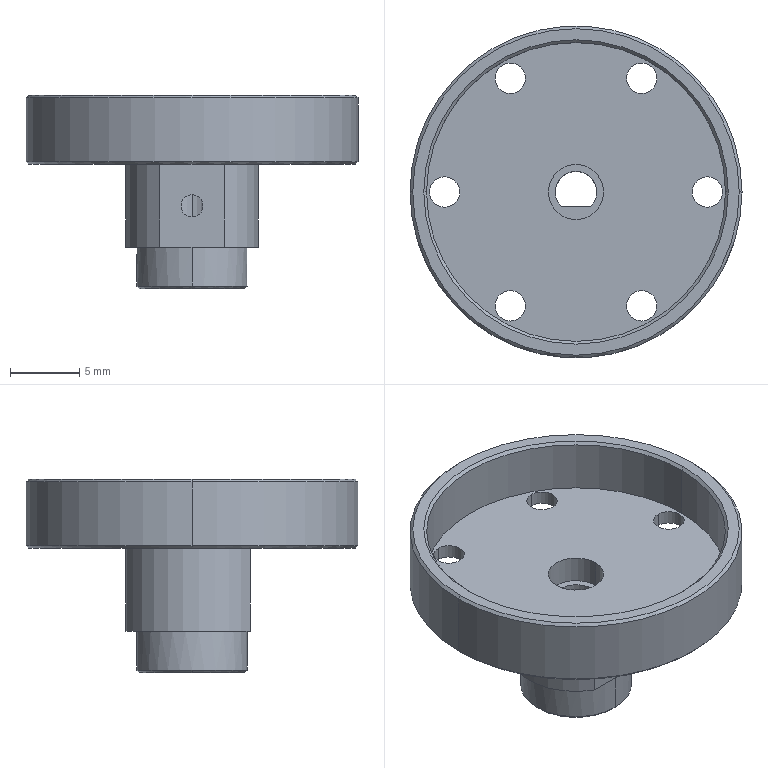NC program | NX | posted with a generic post | part box 24 x 24 x 14 mm
Lines 1 to 1709 of 3647, first 1603 of 1689 lines:
N10 G17 G21 G94 G90
(FLOOR_WALL_COPY , TOOL : D80)
N12 T19 M6
N14 G54
N16 G17 G0 G90 X-55. Y0. S6500 M3
N18 G43 Z30. H19
N20 Z8.
N22 G94 G1 Z5. F1500.
N24 X-52.
N26 X52.
N28 X55.
N30 Z8.
N32 G0 Z30.
N34 X-55.
N36 Z7.
N38 G1 Z4.
N40 X-52.
N42 X52.
N44 X55.
N46 Z7.
N48 G0 Z30.
N50 X-55.
N52 Z6.
N54 G1 Z3.
N56 X-52.
N58 X52.
N60 X55.
N62 Z6.
N64 G0 Z30.
N66 X-55.
N68 Z5.
N70 G1 Z2.
N72 X-52.
N74 X52.
N76 X55.
N78 Z5.
N80 G0 Z30.
N82 X-55.
N84 Z4.
N86 G1 Z1.
N88 X-52.
N90 X52.
N92 X55.
N94 Z4.
N96 G0 Z30.
N98 X-55.
N100 Z3.
N102 G1 Z0.
N104 X-52.
N106 X52.
N108 X55.
N110 Z3.
N112 G0 Z30.
N114 M5
(FLOOR_WALL_2 , TOOL : D10)
N116 T15 M6
N118 G54
N120 G17 G0 G90 X-18.446 Y-1.412 S9500 M3
N122 G43 Z30. H15
N124 Z1.1
N126 G94 G1 Z-0.4 F1000.
N128 X-17.5 Y-0.866
N130 G3 X-17. Y0. R1.
N132 G2 X0. Y17. R17. F2000.
N134 X-17. Y0. R-17.
N136 G1 X-12.
N138 G2 X0. Y12. R12.
N140 X-12. Y0. R-12.
N142 G1 X-9.9
N144 G2 X4.793 Y-8.663 R-9.9
N146 G1 X3.641 Y-9.3
N148 X-3.641
N150 X-4.793 Y-8.663
N152 G2 X-9.9 Y0. R9.9
N154 G3 X-10.4 Y0.866 R1.
N156 G1 Z1.1
N158 G0 X-18.446 Y-1.412 Z0.6
N160 G1 Z-0.9 F1000.
N162 X-17.5 Y-0.866
N164 G3 X-17. Y0. R1.
N166 G2 X0. Y17. R17. F2000.
N168 X-17. Y0. R-17.
N170 G1 X-12.
N172 G2 X0. Y12. R12.
N174 X-12. Y0. R-12.
N176 G1 X-9.9
N178 G2 X4.793 Y-8.663 R-9.9
N180 G1 X3.641 Y-9.3
N182 X-3.641
N184 X-4.793 Y-8.663
N186 G2 X-9.9 Y0. R9.9
N188 G3 X-10.4 Y0.866 R1.
N190 G1 Z0.6
N192 G0 X-18.446 Y-1.412 Z0.1
N194 G1 Z-1.4 F1000.
N196 X-17.5 Y-0.866
N198 G3 X-17. Y0. R1.
N200 G2 X0. Y17. R17. F2000.
N202 X-17. Y0. R-17.
N204 G1 X-12.
N206 G2 X0. Y12. R12.
N208 X-12. Y0. R-12.
N210 G1 X-9.9
N212 G2 X4.793 Y-8.663 R-9.9
N214 G1 X3.641 Y-9.3
N216 X-3.641
N218 X-4.793 Y-8.663
N220 G2 X-9.9 Y0. R9.9
N222 G3 X-10.4 Y0.866 R1.
N224 G1 Z0.1
N226 G0 X-18.446 Y-1.412 Z-0.4
N228 G1 Z-1.9 F1000.
N230 X-17.5 Y-0.866
N232 G3 X-17. Y0. R1.
N234 G2 X0. Y17. R17. F2000.
N236 X-17. Y0. R-17.
N238 G1 X-12.
N240 G2 X0. Y12. R12.
N242 X-12. Y0. R-12.
N244 G1 X-9.9
N246 G2 X4.793 Y-8.663 R-9.9
N248 G1 X3.641 Y-9.3
N250 X-3.641
N252 X-4.793 Y-8.663
N254 G2 X-9.9 Y0. R9.9
N256 G3 X-10.4 Y0.866 R1.
N258 G1 Z-0.4
N260 G0 X-18.446 Y-1.412 Z-0.9
N262 G1 Z-2.4 F1000.
N264 X-17.5 Y-0.866
N266 G3 X-17. Y0. R1.
N268 G2 X0. Y17. R17. F2000.
N270 X-17. Y0. R-17.
N272 G1 X-12.
N274 G2 X0. Y12. R12.
N276 X-12. Y0. R-12.
N278 G1 X-9.9
N280 G2 X4.793 Y-8.663 R-9.9
N282 G1 X3.641 Y-9.3
N284 X-3.641
N286 X-4.793 Y-8.663
N288 G2 X-9.9 Y0. R9.9
N290 G3 X-10.4 Y0.866 R1.
N292 G1 Z-0.9
N294 G0 X-18.446 Y-1.412 Z-1.4
N296 G1 Z-2.9 F1000.
N298 X-17.5 Y-0.866
N300 G3 X-17. Y0. R1.
N302 G2 X0. Y17. R17. F2000.
N304 X-17. Y0. R-17.
N306 G1 X-12.
N308 G2 X0. Y12. R12.
N310 X-12. Y0. R-12.
N312 G1 X-9.9
N314 G2 X4.793 Y-8.663 R-9.9
N316 G1 X3.641 Y-9.3
N318 X-3.641
N320 X-4.793 Y-8.663
N322 G2 X-9.9 Y0. R9.9
N324 G3 X-10.4 Y0.866 R1.
N326 G1 Z-1.4
N328 G0 X-18.446 Y-1.412 Z-1.9
N330 G1 Z-3.4 F1000.
N332 X-17.5 Y-0.866
N334 G3 X-17. Y0. R1.
N336 G2 X0. Y17. R17. F2000.
N338 X-17. Y0. R-17.
N340 G1 X-12.
N342 G2 X0. Y12. R12.
N344 X-12. Y0. R-12.
N346 G1 X-9.9
N348 G2 X4.793 Y-8.663 R-9.9
N350 G1 X3.641 Y-9.3
N352 X-3.641
N354 X-4.793 Y-8.663
N356 G2 X-9.9 Y0. R9.9
N358 G3 X-10.4 Y0.866 R1.
N360 G1 Z-1.9
N362 G0 X-18.446 Y-1.412 Z-2.4
N364 G1 Z-3.9 F1000.
N366 X-17.5 Y-0.866
N368 G3 X-17. Y0. R1.
N370 G2 X0. Y17. R17. F2000.
N372 X-17. Y0. R-17.
N374 G1 X-12.
N376 G2 X0. Y12. R12.
N378 X-12. Y0. R-12.
N380 G1 X-9.9
N382 G2 X4.793 Y-8.663 R-9.9
N384 G1 X3.641 Y-9.3
N386 X-3.641
N388 X-4.793 Y-8.663
N390 G2 X-9.9 Y0. R9.9
N392 G3 X-10.4 Y0.866 R1.
N394 G1 Z-2.4
N396 G0 X-18.446 Y-1.412 Z-2.9
N398 G1 Z-4.4 F1000.
N400 X-17.5 Y-0.866
N402 G3 X-17. Y0. R1.
N404 G2 X0. Y17. R17. F2000.
N406 X-17. Y0. R-17.
N408 G1 X-12.
N410 G2 X0. Y12. R12.
N412 X-12. Y0. R-12.
N414 G1 X-9.9
N416 G2 X4.793 Y-8.663 R-9.9
N418 G1 X3.641 Y-9.3
N420 X-3.641
N422 X-4.793 Y-8.663
N424 G2 X-9.9 Y0. R9.9
N426 G3 X-10.4 Y0.866 R1.
N428 G1 Z-2.9
N430 G0 X-18.446 Y-1.412 Z-3.4
N432 G1 Z-4.9 F1000.
N434 X-17.5 Y-0.866
N436 G3 X-17. Y0. R1.
N438 G2 X0. Y17. R17. F2000.
N440 X-17. Y0. R-17.
N442 G1 X-12.
N444 G2 X0. Y12. R12.
N446 X-12. Y0. R-12.
N448 G1 X-9.9
N450 G2 X4.793 Y-8.663 R-9.9
N452 G1 X3.641 Y-9.3
N454 X-3.641
N456 X-4.793 Y-8.663
N458 G2 X-9.9 Y0. R9.9
N460 G3 X-10.4 Y0.866 R1.
N462 G1 Z-3.4
N464 G0 X-18.446 Y-1.412 Z-3.9
N466 G1 Z-5.4 F1000.
N468 X-17.5 Y-0.866
N470 G3 X-17. Y0. R1.
N472 G2 X0. Y17. R17. F2000.
N474 X-17. Y0. R-17.
N476 G1 X-12.
N478 G2 X0. Y12. R12.
N480 X-12. Y0. R-12.
N482 G1 X-9.9
N484 G2 X4.793 Y-8.663 R-9.9
N486 G1 X3.641 Y-9.3
N488 X-3.641
N490 X-4.793 Y-8.663
N492 G2 X-9.9 Y0. R9.9
N494 G3 X-10.4 Y0.866 R1.
N496 G1 Z-3.9
N498 G0 X-18.446 Y-1.412 Z-4.4
N500 G1 Z-5.9 F1000.
N502 X-17.5 Y-0.866
N504 G3 X-17. Y0. R1.
N506 G2 X0. Y17. R17. F2000.
N508 X-17. Y0. R-17.
N510 G1 X-12.
N512 G2 X0. Y12. R12.
N514 X-12. Y0. R-12.
N516 G1 X-9.9
N518 G2 X4.793 Y-8.663 R-9.9
N520 G1 X3.641 Y-9.3
N522 X-3.641
N524 X-4.793 Y-8.663
N526 G2 X-9.9 Y0. R9.9
N528 G3 X-10.4 Y0.866 R1.
N530 G1 Z-4.4
N532 G0 X-18.446 Y-1.412 Z-4.9
N534 G1 Z-6.4 F1000.
N536 X-17.5 Y-0.866
N538 G3 X-17. Y0. R1.
N540 G2 X0. Y17. R17. F2000.
N542 X-17. Y0. R-17.
N544 G1 X-12.
N546 G2 X0. Y12. R12.
N548 X-12. Y0. R-12.
N550 G1 X-9.9
N552 G2 X4.793 Y-8.663 R-9.9
N554 G1 X3.641 Y-9.3
N556 X-3.641
N558 X-4.793 Y-8.663
N560 G2 X-9.9 Y0. R9.9
N562 G3 X-10.4 Y0.866 R1.
N564 G1 Z-4.9
N566 G0 X-18.446 Y-1.412 Z-5.4
N568 G1 Z-6.9 F1000.
N570 X-17.5 Y-0.866
N572 G3 X-17. Y0. R1.
N574 G2 X0. Y17. R17. F2000.
N576 X-17. Y0. R-17.
N578 G1 X-12.
N580 G2 X0. Y12. R12.
N582 X-12. Y0. R-12.
N584 G1 X-9.9
N586 G2 X4.793 Y-8.663 R-9.9
N588 G1 X3.641 Y-9.3
N590 X-3.641
N592 X-4.793 Y-8.663
N594 G2 X-9.9 Y0. R9.9
N596 G3 X-10.4 Y0.866 R1.
N598 G1 Z-5.4
N600 G0 X-18.446 Y-1.412 Z-5.9
N602 G1 Z-7.4 F1000.
N604 X-17.5 Y-0.866
N606 G3 X-17. Y0. R1.
N608 G2 X0. Y17. R17. F2000.
N610 X-17. Y0. R-17.
N612 G1 X-12.
N614 G2 X0. Y12. R12.
N616 X-12. Y0. R-12.
N618 G1 X-9.9
N620 G2 X4.793 Y-8.663 R-9.9
N622 G1 X3.641 Y-9.3
N624 X-3.641
N626 X-4.793 Y-8.663
N628 G2 X-9.9 Y0. R9.9
N630 G3 X-10.4 Y0.866 R1.
N632 G1 Z-5.9
N634 G0 X-18.446 Y-1.412 Z-6.4
N636 G1 Z-7.9 F1000.
N638 X-17.5 Y-0.866
N640 G3 X-17. Y0. R1.
N642 G2 X0. Y17. R17. F2000.
N644 X-17. Y0. R-17.
N646 G1 X-12.
N648 G2 X0. Y12. R12.
N650 X-12. Y0. R-12.
N652 G1 X-9.9
N654 G2 X4.793 Y-8.663 R-9.9
N656 G1 X3.641 Y-9.3
N658 X-3.641
N660 X-4.793 Y-8.663
N662 G2 X-9.9 Y0. R9.9
N664 G3 X-10.4 Y0.866 R1.
N666 G1 Z-6.4
N668 G0 X-18.446 Y-1.412 Z-6.9
N670 G1 Z-8.4 F1000.
N672 X-17.5 Y-0.866
N674 G3 X-17. Y0. R1.
N676 G2 X0. Y17. R17. F2000.
N678 X-17. Y0. R-17.
N680 G1 X-12.
N682 G2 X0. Y12. R12.
N684 X-12. Y0. R-12.
N686 G1 X-9.9
N688 G2 X4.793 Y-8.663 R-9.9
N690 G1 X3.641 Y-9.3
N692 X-3.641
N694 X-4.793 Y-8.663
N696 G2 X-9.9 Y0. R9.9
N698 G3 X-10.4 Y0.866 R1.
N700 G1 Z-6.9
N702 G0 X-18.446 Y-1.412 Z-7.4
N704 G1 Z-8.9 F1000.
N706 X-17.5 Y-0.866
N708 G3 X-17. Y0. R1.
N710 G2 X0. Y17. R17. F2000.
N712 X-17. Y0. R-17.
N714 G1 X-12.
N716 G2 X0. Y12. R12.
N718 X-12. Y0. R-12.
N720 G1 X-9.9
N722 G2 X4.793 Y-8.663 R-9.9
N724 G1 X3.641 Y-9.3
N726 X-3.641
N728 X-4.793 Y-8.663
N730 G2 X-9.9 Y0. R9.9
N732 G3 X-10.4 Y0.866 R1.
N734 G1 Z-7.4
N736 G0 Z30.
(FLOOR_WALL_2_COPY , TOOL : D10)
N738 X-10.508 Y-1.39
N740 Z1.1
N742 G1 Z-0.4 F1000.
N744 X-9.6 Y-0.866
N746 G3 X-9.1 Y0. R1.
N748 G2 X0. Y9.1 R9.1 F2000.
N750 X-9.1 Y0. R-9.1
N752 G3 X-9.6 Y0.866 R1.
N754 G1 X-10.508 Y1.39
N756 Z1.1
N758 G0 Y-1.39 Z0.6
N760 G1 Z-0.9 F1000.
N762 X-9.6 Y-0.866
N764 G3 X-9.1 Y0. R1.
N766 G2 X0. Y9.1 R9.1 F2000.
N768 X-9.1 Y0. R-9.1
N770 G3 X-9.6 Y0.866 R1.
N772 G1 X-10.508 Y1.39
N774 Z0.6
N776 G0 Y-1.39 Z0.1
N778 G1 Z-1.4 F1000.
N780 X-9.6 Y-0.866
N782 G3 X-9.1 Y0. R1.
N784 G2 X0. Y9.1 R9.1 F2000.
N786 X-9.1 Y0. R-9.1
N788 G3 X-9.6 Y0.866 R1.
N790 G1 X-10.508 Y1.39
N792 Z0.1
N794 G0 Y-1.39 Z-0.4
N796 G1 Z-1.9 F1000.
N798 X-9.6 Y-0.866
N800 G3 X-9.1 Y0. R1.
N802 G2 X0. Y9.1 R9.1 F2000.
N804 X-9.1 Y0. R-9.1
N806 G3 X-9.6 Y0.866 R1.
N808 G1 X-10.508 Y1.39
N810 Z-0.4
N812 G0 Y-1.39 Z-0.9
N814 G1 Z-2.4 F1000.
N816 X-9.6 Y-0.866
N818 G3 X-9.1 Y0. R1.
N820 G2 X0. Y9.1 R9.1 F2000.
N822 X-9.1 Y0. R-9.1
N824 G3 X-9.6 Y0.866 R1.
N826 G1 X-10.508 Y1.39
N828 Z-0.9
N830 G0 Y-1.39 Z-1.4
N832 G1 Z-2.9 F1000.
N834 X-9.6 Y-0.866
N836 G3 X-9.1 Y0. R1.
N838 G2 X0. Y9.1 R9.1 F2000.
N840 X-9.1 Y0. R-9.1
N842 G3 X-9.6 Y0.866 R1.
N844 G1 X-10.508 Y1.39
N846 Z-1.4
N848 G0 Z30.
N850 M5
(FLOOR_WALL_1_COPY , TOOL : D10JING)
N852 T14 M6
N854 G54
N856 G17 G0 G90 X2.021 Y-12.2 S9500 M3
N858 G43 Z30. H14
N860 Z-6.
N862 G94 G1 Z-9. F1250.
N864 X0.866 Y-10.2
N866 G3 X0. Y-9.7 R1.
N868 G1 X-3.615
N870 G2 X-3.857 Y-9.638 R0.5
N872 G1 X-4.986 Y-9.013
N874 G2 X4.986 Y-9.013 R-10.3
N876 G1 X3.857 Y-9.638
N878 G2 X3.615 Y-9.7 R0.5
N880 G1 X0.
N882 X0.866
N884 G3 X0. Y-9.2 R1.
N886 G1 X-3.615
N888 X-4.744 Y-8.575
N890 G2 X4.744 Y-8.575 R-9.8
N892 G1 X3.615 Y-9.2
N894 X0.
N896 G3 X-0.866 Y-9.7 R1.
N898 G1 X-2.598 Y-12.7
N900 Z-6.
N902 G0 Z30.
N904 M5
(DRILLING , TOOL : D6A45)
N906 T01 M6
N908 G54
N910 G17 G0 G90 X2.75 Y0. S5000 M3
N912 G43 Z30. H1
N914 G94 G81 G98 Z-0.725 F350. R3.
N916 X-2.75
N918 G80
N920 G0 X-2.75 Y0. Z30.
(DRILLING_COPY , TOOL : D6A45)
N922 X9.5
N924 G81 Z-10.2 F350. R-6.
N926 X4.75 Y-8.227
N928 X-4.75
N930 X-9.5 Y0.
N932 X-4.75 Y8.227
N934 X4.75
N936 G80
N938 G0 X4.75 Y8.227 Z30.
N940 M5
(DRILLING_COPY_1 , TOOL : 1.25ZT)
N942 T17 M6
N944 G54
N946 G17 G0 G90 X2.75 Y0. S2000 M3
N948 G43 Z30. H17
N950 G94 G83 G98 Z-4.626 F120. Q1. R3.
N952 X-2.75
N954 G80
N956 G0 X-2.75 Y0. Z30.
N958 M5
(DRILLING_COPY_1_COPY , TOOL : 2.2ZT)
N960 T18 M6
N962 G54
N964 G17 G0 G90 X-4.75 Y8.227 S2000 M3
N966 G43 Z30. H18
N968 G94 G83 G98 Z-12.161 F120. Q1. R-6.
N970 Y-8.227
N972 X9.5 Y0.
N974 X4.75 Y-8.227
N976 X-9.5 Y0.
N978 X4.75 Y8.227
N980 G80
N982 G0 X4.75 Y8.227 Z30.
N984 M5
(ZLEVEL_PROFILE , TOOL : D2)
N986 T24 M6
N988 G54
N990 G17 G0 G90 X-0.272 Y0.298 S9500 M3
N992 G43 Z30. H24
N994 Z0.5
N996 G94 G1 X-0.35 Y0.213 Z0.494 F1000.
N998 X-0.379 Y0.128 Z0.489
N1000 X-0.389 Y0.05 Z0.485
N1002 X0.389 Z0.444
N1004 X0.379 Y0.127 Z0.44
N1006 X0.351 Y0.212 Z0.436
N1008 X0.238 Y0.334 Z0.427
N1010 X0.086 Y0.401 Z0.418
N1012 X-0.094 Y0.399 Z0.409
N1014 X-0.241 Y0.332 Z0.4
N1016 X-0.35 Y0.213 Z0.392
N1018 X-0.379 Y0.128 Z0.387
N1020 X-0.389 Y0.05 Z0.383
N1022 X0.389 Z0.342
N1024 X0.379 Y0.127 Z0.338
N1026 X0.351 Y0.212 Z0.333
N1028 X0.238 Y0.334 Z0.325
N1030 X0.086 Y0.401 Z0.316
N1032 X-0.094 Y0.399 Z0.307
N1034 X-0.241 Y0.332 Z0.298
N1036 X-0.35 Y0.213 Z0.29
N1038 X-0.379 Y0.128 Z0.285
N1040 X-0.389 Y0.05 Z0.281
N1042 X0.389 Z0.24
N1044 X0.379 Y0.127 Z0.236
N1046 X0.351 Y0.212 Z0.231
N1048 X0.238 Y0.334 Z0.223
N1050 X0.086 Y0.401 Z0.214
N1052 X-0.094 Y0.399 Z0.204
N1054 X-0.241 Y0.332 Z0.196
N1056 X-0.35 Y0.213 Z0.187
N1058 X-0.379 Y0.128 Z0.183
N1060 X-0.389 Y0.05 Z0.179
N1062 X0.389 Z0.138
N1064 X0.379 Y0.127 Z0.134
N1066 X0.351 Y0.212 Z0.129
N1068 X0.238 Y0.334 Z0.12
N1070 X0.086 Y0.401 Z0.112
N1072 X-0.094 Y0.399 Z0.102
N1074 X-0.241 Y0.332 Z0.094
N1076 X-0.35 Y0.213 Z0.085
N1078 X-0.379 Y0.128 Z0.081
N1080 X-0.389 Y0.05 Z0.077
N1082 X0.389 Z0.036
N1084 X0.379 Y0.127 Z0.032
N1086 X0.351 Y0.212 Z0.027
N1088 X0.238 Y0.334 Z0.018
N1090 X0.086 Y0.401 Z0.01
N1092 X-0.094 Y0.399 Z0.
N1094 X-0.241 Y0.332 Z-0.008
N1096 X-0.35 Y0.213 Z-0.017
N1098 X-0.379 Y0.128 Z-0.022
N1100 X-0.389 Y0.05 Z-0.026
N1102 X0.389 Z-0.066
N1104 X0.379 Y0.127 Z-0.07
N1106 X0.351 Y0.212 Z-0.075
N1108 X0.238 Y0.334 Z-0.084
N1110 X0.086 Y0.401 Z-0.093
N1112 X-0.094 Y0.399 Z-0.102
N1114 X-0.241 Y0.332 Z-0.11
N1116 X-0.35 Y0.213 Z-0.119
N1118 X-0.379 Y0.128 Z-0.124
N1120 X-0.389 Y0.05 Z-0.128
N1122 X0. Z-0.148
N1124 X0.389
N1126 X0.379 Y0.127
N1128 G3 X-0.379 Y0.128 R0.4
N1130 G1 X-0.389 Y0.05
N1132 X0.
N1134 X0.181 Z-0.167
N1136 X0.387 Y0.06 Z-0.181
N1138 X0.379 Y0.107 Z-0.185
N1140 X0.359 Y0.157 Z-0.194
N1142 X0.332 Y0.21 Z-0.204
N1144 X0.224 Y0.324 Z-0.222
N1146 X0.172 Y0.354 Z-0.228
N1148 X0.145 Y0.366 Z-0.231
N1150 X0.117 Y0.375 Z-0.235
N1152 X0.059 Y0.388 Z-0.241
N1154 X-0.012 Y0.394 Z-0.248
N1156 X-0.071 Y0.387 Z-0.254
N1158 X-0.117 Y0.375 Z-0.259
N1160 X-0.184 Y0.347 Z-0.267
N1162 X-0.235 Y0.317 Z-0.273
N1164 X-0.269 Y0.286 Z-0.278
N1166 X-0.327 Y0.218 Z-0.287
N1168 X-0.374 Y0.142 Z-0.296
N1170 X-0.379 Y0.128
N1172 X-0.389 Y0.05
N1174 X0.
N1176 X0.181 Z-0.315
N1178 X0.387 Y0.06 Z-0.329
N1180 X0.379 Y0.107 Z-0.333
N1182 X0.359 Y0.157 Z-0.342
N1184 X0.332 Y0.21 Z-0.352
N1186 X0.224 Y0.324 Z-0.37
N1188 X0.172 Y0.354 Z-0.377
N1190 X0.145 Y0.366 Z-0.38
N1192 X0.117 Y0.375 Z-0.383
N1194 X0.059 Y0.388 Z-0.389
N1196 X-0.012 Y0.394 Z-0.396
N1198 X-0.071 Y0.387 Z-0.402
N1200 X-0.117 Y0.375 Z-0.407
N1202 X-0.184 Y0.347 Z-0.415
N1204 X-0.235 Y0.317 Z-0.421
N1206 X-0.269 Y0.286 Z-0.426
N1208 X-0.327 Y0.218 Z-0.435
N1210 X-0.374 Y0.142 Z-0.444
N1212 X-0.379 Y0.128
N1214 X-0.389 Y0.05
N1216 X0.
N1218 X0.181 Z-0.463
N1220 X0.387 Y0.06 Z-0.477
N1222 X0.379 Y0.107 Z-0.481
N1224 X0.359 Y0.157 Z-0.491
N1226 X0.332 Y0.21 Z-0.5
N1228 X0.224 Y0.324 Z-0.519
N1230 X0.172 Y0.354 Z-0.525
N1232 X0.145 Y0.366 Z-0.528
N1234 X0.117 Y0.375 Z-0.531
N1236 X0.059 Y0.388 Z-0.537
N1238 X-0.012 Y0.394 Z-0.544
N1240 X-0.071 Y0.387 Z-0.551
N1242 X-0.117 Y0.375 Z-0.556
N1244 X-0.184 Y0.347 Z-0.563
N1246 X-0.235 Y0.317 Z-0.569
N1248 X-0.269 Y0.286 Z-0.574
N1250 X-0.327 Y0.218 Z-0.583
N1252 X-0.374 Y0.142 Z-0.593
N1254 X-0.379 Y0.128
N1256 X-0.389 Y0.05
N1258 X0.
N1260 X0.181 Z-0.611
N1262 X0.387 Y0.06 Z-0.626
N1264 X0.379 Y0.107 Z-0.63
N1266 X0.359 Y0.157 Z-0.639
N1268 X0.332 Y0.21 Z-0.648
N1270 X0.224 Y0.324 Z-0.667
N1272 X0.172 Y0.354 Z-0.673
N1274 X0.145 Y0.366 Z-0.676
N1276 X0.117 Y0.375 Z-0.679
N1278 X0.059 Y0.388 Z-0.685
N1280 X-0.012 Y0.394 Z-0.693
N1282 X-0.071 Y0.387 Z-0.699
N1284 X-0.117 Y0.375 Z-0.704
N1286 X-0.184 Y0.347 Z-0.711
N1288 X-0.235 Y0.317 Z-0.717
N1290 X-0.269 Y0.286 Z-0.722
N1292 X-0.327 Y0.218 Z-0.731
N1294 X-0.374 Y0.142 Z-0.741
N1296 X-0.379 Y0.128
N1298 X-0.389 Y0.05
N1300 X0.
N1302 X0.181 Z-0.759
N1304 X0.387 Y0.06 Z-0.774
N1306 X0.379 Y0.107 Z-0.778
N1308 X0.359 Y0.157 Z-0.787
N1310 X0.332 Y0.21 Z-0.796
N1312 X0.224 Y0.324 Z-0.815
N1314 X0.172 Y0.354 Z-0.821
N1316 X0.145 Y0.366 Z-0.824
N1318 X0.117 Y0.375 Z-0.827
N1320 X0.059 Y0.388 Z-0.833
N1322 X-0.012 Y0.394 Z-0.841
N1324 X-0.071 Y0.387 Z-0.847
N1326 X-0.117 Y0.375 Z-0.852
N1328 X-0.184 Y0.347 Z-0.859
N1330 X-0.235 Y0.317 Z-0.866
N1332 X-0.269 Y0.286 Z-0.87
N1334 X-0.327 Y0.218 Z-0.88
N1336 X-0.374 Y0.142 Z-0.889
N1338 X-0.379 Y0.128
N1340 X-0.389 Y0.05
N1342 X0.
N1344 X0.181 Z-0.907
N1346 X0.387 Y0.06 Z-0.922
N1348 X0.379 Y0.107 Z-0.926
N1350 X0.359 Y0.157 Z-0.935
N1352 X0.332 Y0.21 Z-0.944
N1354 X0.224 Y0.324 Z-0.963
N1356 X0.172 Y0.354 Z-0.969
N1358 X0.145 Y0.366 Z-0.972
N1360 X0.117 Y0.375 Z-0.975
N1362 X0.059 Y0.388 Z-0.981
N1364 X-0.012 Y0.394 Z-0.989
N1366 X-0.071 Y0.387 Z-0.995
N1368 X-0.117 Y0.375 Z-1.
N1370 X-0.184 Y0.347 Z-1.008
N1372 X-0.235 Y0.317 Z-1.014
N1374 X-0.269 Y0.286 Z-1.019
N1376 X-0.327 Y0.218 Z-1.028
N1378 X-0.374 Y0.142 Z-1.037
N1380 X-0.379 Y0.128
N1382 X-0.389 Y0.05
N1384 X0.
N1386 X0.181 Z-1.056
N1388 X0.387 Y0.06 Z-1.07
N1390 X0.379 Y0.107 Z-1.074
N1392 X0.359 Y0.157 Z-1.083
N1394 X0.332 Y0.21 Z-1.092
N1396 X0.224 Y0.324 Z-1.111
N1398 X0.172 Y0.354 Z-1.117
N1400 X0.145 Y0.366 Z-1.12
N1402 X0.117 Y0.375 Z-1.123
N1404 X0.059 Y0.388 Z-1.13
N1406 X-0.012 Y0.394 Z-1.137
N1408 X-0.071 Y0.387 Z-1.143
N1410 X-0.117 Y0.375 Z-1.148
N1412 X-0.184 Y0.347 Z-1.156
N1414 X-0.235 Y0.317 Z-1.162
N1416 X-0.269 Y0.286 Z-1.167
N1418 X-0.327 Y0.218 Z-1.176
N1420 X-0.374 Y0.142 Z-1.185
N1422 X-0.379 Y0.128
N1424 X-0.389 Y0.05
N1426 X0.
N1428 X0.181 Z-1.204
N1430 X0.387 Y0.06 Z-1.218
N1432 X0.379 Y0.107 Z-1.222
N1434 X0.359 Y0.157 Z-1.231
N1436 X0.332 Y0.21 Z-1.241
N1438 X0.224 Y0.324 Z-1.259
N1440 X0.172 Y0.354 Z-1.265
N1442 X0.145 Y0.366 Z-1.268
N1444 X0.117 Y0.375 Z-1.272
N1446 X0.059 Y0.388 Z-1.278
N1448 X-0.012 Y0.394 Z-1.285
N1450 X-0.071 Y0.387 Z-1.291
N1452 X-0.117 Y0.375 Z-1.296
N1454 X-0.184 Y0.347 Z-1.304
N1456 X-0.235 Y0.317 Z-1.31
N1458 X-0.269 Y0.286 Z-1.315
N1460 X-0.327 Y0.218 Z-1.324
N1462 X-0.374 Y0.142 Z-1.333
N1464 X-0.379 Y0.128
N1466 X-0.389 Y0.05
N1468 X0.
N1470 X0.181 Z-1.352
N1472 X0.387 Y0.06 Z-1.366
N1474 X0.379 Y0.107 Z-1.37
N1476 X0.359 Y0.157 Z-1.379
N1478 X0.332 Y0.21 Z-1.389
N1480 X0.224 Y0.324 Z-1.407
N1482 X0.172 Y0.354 Z-1.414
N1484 X0.145 Y0.366 Z-1.417
N1486 X0.117 Y0.375 Z-1.42
N1488 X0.059 Y0.388 Z-1.426
N1490 X-0.012 Y0.394 Z-1.433
N1492 X-0.071 Y0.387 Z-1.439
N1494 X-0.117 Y0.375 Z-1.444
N1496 X-0.184 Y0.347 Z-1.452
N1498 X-0.235 Y0.317 Z-1.458
N1500 X-0.269 Y0.286 Z-1.463
N1502 X-0.327 Y0.218 Z-1.472
N1504 X-0.374 Y0.142 Z-1.481
N1506 X-0.379 Y0.128
N1508 X-0.389 Y0.05
N1510 X0.
N1512 X0.181 Z-1.5
N1514 X0.387 Y0.06 Z-1.514
N1516 X0.379 Y0.107 Z-1.518
N1518 X0.359 Y0.157 Z-1.528
N1520 X0.332 Y0.21 Z-1.537
N1522 X0.224 Y0.324 Z-1.556
N1524 X0.172 Y0.354 Z-1.562
N1526 X0.145 Y0.366 Z-1.565
N1528 X0.117 Y0.375 Z-1.568
N1530 X0.059 Y0.388 Z-1.574
N1532 X-0.012 Y0.394 Z-1.581
N1534 X-0.071 Y0.387 Z-1.588
N1536 X-0.117 Y0.375 Z-1.593
N1538 X-0.184 Y0.347 Z-1.6
N1540 X-0.235 Y0.317 Z-1.606
N1542 X-0.269 Y0.286 Z-1.611
N1544 X-0.327 Y0.218 Z-1.62
N1546 X-0.374 Y0.142 Z-1.63
N1548 X-0.379 Y0.128
N1550 X-0.389 Y0.05
N1552 X0.
N1554 X0.181 Z-1.648
N1556 X0.387 Y0.06 Z-1.663
N1558 X0.379 Y0.107 Z-1.667
N1560 X0.359 Y0.157 Z-1.676
N1562 X0.332 Y0.21 Z-1.685
N1564 X0.224 Y0.324 Z-1.704
N1566 X0.172 Y0.354 Z-1.71
N1568 X0.145 Y0.366 Z-1.713
N1570 X0.117 Y0.375 Z-1.716
N1572 X0.059 Y0.388 Z-1.722
N1574 X-0.012 Y0.394 Z-1.73
N1576 X-0.071 Y0.387 Z-1.736
N1578 X-0.117 Y0.375 Z-1.741
N1580 X-0.184 Y0.347 Z-1.748
N1582 X-0.235 Y0.317 Z-1.754
N1584 X-0.269 Y0.286 Z-1.759
N1586 X-0.327 Y0.218 Z-1.769
N1588 X-0.374 Y0.142 Z-1.778
N1590 X-0.379 Y0.128
N1592 X-0.389 Y0.05
N1594 X0.
N1596 X0.181 Z-1.796
N1598 X0.387 Y0.06 Z-1.811
N1600 X0.379 Y0.107 Z-1.815
N1602 X0.359 Y0.157 Z-1.824
N1604 X0.332 Y0.21 Z-1.833
N1606 X0.224 Y0.324 Z-1.852
N1608 X0.172 Y0.354 Z-1.858
N1610 X0.145 Y0.366 Z-1.861
N1612 X0.117 Y0.375 Z-1.864
N1614 X0.059 Y0.388 Z-1.87
N1616 X-0.012 Y0.394 Z-1.878
N1618 X-0.071 Y0.387 Z-1.884
N1620 X-0.117 Y0.375 Z-1.889
N1622 X-0.184 Y0.347 Z-1.896
N1624 X-0.235 Y0.317 Z-1.903
N1626 X-0.269 Y0.286 Z-1.907
N1628 X-0.327 Y0.218 Z-1.917
N1630 X-0.374 Y0.142 Z-1.926
N1632 X-0.379 Y0.128
N1634 X-0.389 Y0.05
N1636 X0.
N1638 X0.181 Z-1.944
N1640 X0.387 Y0.06 Z-1.959
N1642 X0.379 Y0.107 Z-1.963
N1644 X0.359 Y0.157 Z-1.972
N1646 X0.332 Y0.21 Z-1.981
N1648 X0.224 Y0.324 Z-2.
N1650 X0.172 Y0.354 Z-2.006
N1652 X0.145 Y0.366 Z-2.009
N1654 X0.117 Y0.375 Z-2.012
N1656 X0.059 Y0.388 Z-2.019
N1658 X-0.012 Y0.394 Z-2.026
N1660 X-0.071 Y0.387 Z-2.032
N1662 X-0.117 Y0.375 Z-2.037
N1664 X-0.184 Y0.347 Z-2.045
N1666 X-0.235 Y0.317 Z-2.051
N1668 X-0.269 Y0.286 Z-2.056
N1670 X-0.327 Y0.218 Z-2.065
N1672 X-0.374 Y0.142 Z-2.074
N1674 X-0.379 Y0.128
N1676 X-0.389 Y0.05
N1678 X0.
N1680 X0.181 Z-2.093
N1682 X0.387 Y0.06 Z-2.107
N1684 X0.379 Y0.107 Z-2.111
N1686 X0.359 Y0.157 Z-2.12
N1688 X0.332 Y0.21 Z-2.13
N1690 X0.224 Y0.324 Z-2.148
N1692 X0.172 Y0.354 Z-2.154
N1694 X0.145 Y0.366 Z-2.157
N1696 X0.117 Y0.375 Z-2.16
N1698 X0.059 Y0.388 Z-2.167
N1700 X-0.012 Y0.394 Z-2.174
N1702 X-0.071 Y0.387 Z-2.18
N1704 X-0.117 Y0.375 Z-2.185
N1706 X-0.184 Y0.347 Z-2.193
N1708 X-0.235 Y0.317 Z-2.199
N1710 X-0.269 Y0.286 Z-2.204
N1712 X-0.327 Y0.218 Z-2.213
N1714 X-0.374 Y0.142 Z-2.222
N1716 X-0.379 Y0.128
N1718 X-0.389 Y0.05
N1720 X0.
N1722 X0.181 Z-2.241
N1724 X0.387 Y0.06 Z-2.255
N1726 X0.379 Y0.107 Z-2.259
N1728 X0.359 Y0.157 Z-2.268
N1730 X0.332 Y0.21 Z-2.278
N1732 X0.224 Y0.324 Z-2.296
N1734 X0.172 Y0.354 Z-2.302
N1736 X0.145 Y0.366 Z-2.306
N1738 X0.117 Y0.375 Z-2.309
N1740 X0.059 Y0.388 Z-2.315
N1742 X-0.012 Y0.394 Z-2.322
N1744 X-0.071 Y0.387 Z-2.328
N1746 X-0.117 Y0.375 Z-2.333
N1748 X-0.184 Y0.347 Z-2.341
N1750 X-0.235 Y0.317 Z-2.347
N1752 X-0.269 Y0.286 Z-2.352
N1754 X-0.327 Y0.218 Z-2.361
N1756 X-0.374 Y0.142 Z-2.37
N1758 X-0.379 Y0.128
N1760 X-0.389 Y0.05
N1762 X0.
N1764 X0.181 Z-2.389
N1766 X0.387 Y0.06 Z-2.403
N1768 X0.379 Y0.107 Z-2.407
N1770 X0.359 Y0.157 Z-2.417
N1772 X0.332 Y0.21 Z-2.426
N1774 X0.224 Y0.324 Z-2.444
N1776 X0.172 Y0.354 Z-2.451
N1778 X0.145 Y0.366 Z-2.454
N1780 X0.117 Y0.375 Z-2.457
N1782 X0.059 Y0.388 Z-2.463
N1784 X-0.012 Y0.394 Z-2.47
N1786 X-0.071 Y0.387 Z-2.476
N1788 X-0.117 Y0.375 Z-2.481
N1790 X-0.184 Y0.347 Z-2.489
N1792 X-0.235 Y0.317 Z-2.495
N1794 X-0.269 Y0.286 Z-2.5
N1796 X-0.327 Y0.218 Z-2.509
N1798 X-0.374 Y0.142 Z-2.519
N1800 X-0.379 Y0.128
N1802 X-0.389 Y0.05
N1804 X0.
N1806 X0.181 Z-2.537
N1808 X0.387 Y0.06 Z-2.551
N1810 X0.379 Y0.107 Z-2.555
N1812 X0.359 Y0.157 Z-2.565
N1814 X0.332 Y0.21 Z-2.574
N1816 X0.224 Y0.324 Z-2.593
N1818 X0.172 Y0.354 Z-2.599
N1820 X0.145 Y0.366 Z-2.602
N1822 X0.117 Y0.375 Z-2.605
N1824 X0.059 Y0.388 Z-2.611
N1826 X-0.012 Y0.394 Z-2.618
N1828 X-0.071 Y0.387 Z-2.625
N1830 X-0.117 Y0.375 Z-2.63
N1832 X-0.184 Y0.347 Z-2.637
N1834 X-0.235 Y0.317 Z-2.643
N1836 X-0.269 Y0.286 Z-2.648
N1838 X-0.327 Y0.218 Z-2.657
N1840 X-0.374 Y0.142 Z-2.667
N1842 X-0.379 Y0.128
N1844 X-0.389 Y0.05
N1846 X0.
N1848 X0.181 Z-2.685
N1850 X0.387 Y0.06 Z-2.7
N1852 X0.379 Y0.107 Z-2.704
N1854 X0.359 Y0.157 Z-2.713
N1856 X0.332 Y0.21 Z-2.722
N1858 X0.224 Y0.324 Z-2.741
N1860 X0.172 Y0.354 Z-2.747
N1862 X0.145 Y0.366 Z-2.75
N1864 X0.117 Y0.375 Z-2.753
N1866 X0.059 Y0.388 Z-2.759
N1868 X-0.012 Y0.394 Z-2.767
N1870 X-0.071 Y0.387 Z-2.773
N1872 X-0.117 Y0.375 Z-2.778
N1874 X-0.184 Y0.347 Z-2.785
N1876 X-0.235 Y0.317 Z-2.791
N1878 X-0.269 Y0.286 Z-2.796
N1880 X-0.327 Y0.218 Z-2.806
N1882 X-0.374 Y0.142 Z-2.815
N1884 X-0.379 Y0.128
N1886 X-0.389 Y0.05
N1888 X0.
N1890 X0.181 Z-2.833
N1892 X0.387 Y0.06 Z-2.848
N1894 X0.379 Y0.107 Z-2.852
N1896 X0.359 Y0.157 Z-2.861
N1898 X0.332 Y0.21 Z-2.87
N1900 X0.224 Y0.324 Z-2.889
N1902 X0.172 Y0.354 Z-2.895
N1904 X0.145 Y0.366 Z-2.898
N1906 X0.117 Y0.375 Z-2.901
N1908 X0.059 Y0.388 Z-2.907
N1910 X-0.012 Y0.394 Z-2.915
N1912 X-0.071 Y0.387 Z-2.921
N1914 X-0.117 Y0.375 Z-2.926
N1916 X-0.184 Y0.347 Z-2.933
N1918 X-0.235 Y0.317 Z-2.94
N1920 X-0.269 Y0.286 Z-2.944
N1922 X-0.327 Y0.218 Z-2.954
N1924 X-0.374 Y0.142 Z-2.963
N1926 X-0.379 Y0.128
N1928 X-0.389 Y0.05
N1930 X0.
N1932 X0.181 Z-2.981
N1934 X0.387 Y0.06 Z-2.996
N1936 X0.379 Y0.107 Z-3.
N1938 X0.359 Y0.157 Z-3.009
N1940 X0.332 Y0.21 Z-3.018
N1942 X0.224 Y0.324 Z-3.037
N1944 X0.172 Y0.354 Z-3.043
N1946 X0.145 Y0.366 Z-3.046
N1948 X0.117 Y0.375 Z-3.049
N1950 X0.059 Y0.388 Z-3.056
N1952 X-0.012 Y0.394 Z-3.063
N1954 X-0.071 Y0.387 Z-3.069
N1956 X-0.117 Y0.375 Z-3.074
N1958 X-0.184 Y0.347 Z-3.082
N1960 X-0.235 Y0.317 Z-3.088
N1962 X-0.269 Y0.286 Z-3.093
N1964 X-0.327 Y0.218 Z-3.102
N1966 X-0.374 Y0.142 Z-3.111
N1968 X-0.379 Y0.128
N1970 X-0.389 Y0.05
N1972 X0.
N1974 X0.181 Z-3.13
N1976 X0.387 Y0.06 Z-3.144
N1978 X0.379 Y0.107 Z-3.148
N1980 X0.359 Y0.157 Z-3.157
N1982 X0.332 Y0.21 Z-3.167
N1984 X0.224 Y0.324 Z-3.185
N1986 X0.172 Y0.354 Z-3.191
N1988 X0.145 Y0.366 Z-3.194
N1990 X0.117 Y0.375 Z-3.198
N1992 X0.059 Y0.388 Z-3.204
N1994 X-0.012 Y0.394 Z-3.211
N1996 X-0.071 Y0.387 Z-3.217
N1998 X-0.117 Y0.375 Z-3.222
N2000 X-0.184 Y0.347 Z-3.23
N2002 X-0.235 Y0.317 Z-3.236
N2004 X-0.269 Y0.286 Z-3.241
N2006 X-0.327 Y0.218 Z-3.25
N2008 X-0.374 Y0.142 Z-3.259
N2010 X-0.379 Y0.128
N2012 X-0.389 Y0.05
N2014 X0.
N2016 X0.181 Z-3.278
N2018 X0.387 Y0.06 Z-3.292
N2020 X0.379 Y0.107 Z-3.296
N2022 X0.359 Y0.157 Z-3.305
N2024 X0.332 Y0.21 Z-3.315
N2026 X0.224 Y0.324 Z-3.333
N2028 X0.172 Y0.354 Z-3.339
N2030 X0.145 Y0.366 Z-3.343
N2032 X0.117 Y0.375 Z-3.346
N2034 X0.059 Y0.388 Z-3.352
N2036 X-0.012 Y0.394 Z-3.359
N2038 X-0.071 Y0.387 Z-3.365
N2040 X-0.117 Y0.375 Z-3.37
N2042 X-0.184 Y0.347 Z-3.378
N2044 X-0.235 Y0.317 Z-3.384
N2046 X-0.269 Y0.286 Z-3.389
N2048 X-0.327 Y0.218 Z-3.398
N2050 X-0.374 Y0.142 Z-3.407
N2052 X-0.379 Y0.128
N2054 X-0.389 Y0.05
N2056 X0.
N2058 X0.181 Z-3.426
N2060 X0.387 Y0.06 Z-3.44
N2062 X0.379 Y0.107 Z-3.444
N2064 X0.359 Y0.157 Z-3.454
N2066 X0.332 Y0.21 Z-3.463
N2068 X0.224 Y0.324 Z-3.481
N2070 X0.172 Y0.354 Z-3.488
N2072 X0.145 Y0.366 Z-3.491
N2074 X0.117 Y0.375 Z-3.494
N2076 X0.059 Y0.388 Z-3.5
N2078 X-0.012 Y0.394 Z-3.507
N2080 X-0.071 Y0.387 Z-3.514
N2082 X-0.117 Y0.375 Z-3.519
N2084 X-0.184 Y0.347 Z-3.526
N2086 X-0.235 Y0.317 Z-3.532
N2088 X-0.269 Y0.286 Z-3.537
N2090 X-0.327 Y0.218 Z-3.546
N2092 X-0.374 Y0.142 Z-3.556
N2094 X-0.379 Y0.128
N2096 X-0.389 Y0.05
N2098 X0.
N2100 X0.181 Z-3.574
N2102 X0.387 Y0.06 Z-3.588
N2104 X0.379 Y0.107 Z-3.592
N2106 X0.359 Y0.157 Z-3.602
N2108 X0.332 Y0.21 Z-3.611
N2110 X0.224 Y0.324 Z-3.63
N2112 X0.172 Y0.354 Z-3.636
N2114 X0.145 Y0.366 Z-3.639
N2116 X0.117 Y0.375 Z-3.642
N2118 X0.059 Y0.388 Z-3.648
N2120 X-0.012 Y0.394 Z-3.655
N2122 X-0.071 Y0.387 Z-3.662
N2124 X-0.117 Y0.375 Z-3.667
N2126 X-0.184 Y0.347 Z-3.674
N2128 X-0.235 Y0.317 Z-3.68
N2130 X-0.269 Y0.286 Z-3.685
N2132 X-0.327 Y0.218 Z-3.694
N2134 X-0.374 Y0.142 Z-3.704
N2136 X-0.379 Y0.128
N2138 X-0.389 Y0.05
N2140 X0.
N2142 X0.181 Z-3.722
N2144 X0.387 Y0.06 Z-3.737
N2146 X0.379 Y0.107 Z-3.741
N2148 X0.359 Y0.157 Z-3.75
N2150 X0.332 Y0.21 Z-3.759
N2152 X0.224 Y0.324 Z-3.778
N2154 X0.172 Y0.354 Z-3.784
N2156 X0.145 Y0.366 Z-3.787
N2158 X0.117 Y0.375 Z-3.79
N2160 X0.059 Y0.388 Z-3.796
N2162 X-0.012 Y0.394 Z-3.804
N2164 X-0.071 Y0.387 Z-3.81
N2166 X-0.117 Y0.375 Z-3.815
N2168 X-0.184 Y0.347 Z-3.822
N2170 X-0.235 Y0.317 Z-3.829
N2172 X-0.269 Y0.286 Z-3.833
N2174 X-0.327 Y0.218 Z-3.843
N2176 X-0.374 Y0.142 Z-3.852
N2178 X-0.379 Y0.128
N2180 X-0.389 Y0.05
N2182 X0.
N2184 X0.181 Z-3.87
N2186 X0.387 Y0.06 Z-3.885
N2188 X0.379 Y0.107 Z-3.889
N2190 X0.359 Y0.157 Z-3.898
N2192 X0.332 Y0.21 Z-3.907
N2194 X0.224 Y0.324 Z-3.926
N2196 X0.172 Y0.354 Z-3.932
N2198 X0.145 Y0.366 Z-3.935
N2200 X0.117 Y0.375 Z-3.938
N2202 X0.059 Y0.388 Z-3.944
N2204 X-0.012 Y0.394 Z-3.952
N2206 X-0.071 Y0.387 Z-3.958
N2208 X-0.117 Y0.375 Z-3.963
N2210 X-0.184 Y0.347 Z-3.97
N2212 X-0.235 Y0.317 Z-3.977
N2214 X-0.269 Y0.286 Z-3.981
N2216 X-0.327 Y0.218 Z-3.991
N2218 X-0.374 Y0.142 Z-4.
N2220 X-0.379 Y0.128
N2222 X-0.389 Y0.05
N2224 X0.
N2226 X0.181 Z-4.019
N2228 X0.387 Y0.06 Z-4.033
N2230 X0.379 Y0.107 Z-4.037
N2232 X0.359 Y0.157 Z-4.046
N2234 X0.332 Y0.21 Z-4.055
N2236 X0.224 Y0.324 Z-4.074
N2238 X0.172 Y0.354 Z-4.08
N2240 X0.145 Y0.366 Z-4.083
N2242 X0.117 Y0.375 Z-4.086
N2244 X0.059 Y0.388 Z-4.093
N2246 X-0.012 Y0.394 Z-4.1
N2248 X-0.071 Y0.387 Z-4.106
N2250 X-0.117 Y0.375 Z-4.111
N2252 X-0.184 Y0.347 Z-4.119
N2254 X-0.235 Y0.317 Z-4.125
N2256 X-0.269 Y0.286 Z-4.13
N2258 X-0.327 Y0.218 Z-4.139
N2260 X-0.374 Y0.142 Z-4.148
N2262 X-0.379 Y0.128
N2264 X-0.389 Y0.05
N2266 X0.
N2268 X0.181 Z-4.167
N2270 X0.387 Y0.06 Z-4.181
N2272 X0.379 Y0.107 Z-4.185
N2274 X0.359 Y0.157 Z-4.194
N2276 X0.332 Y0.21 Z-4.204
N2278 X0.224 Y0.324 Z-4.222
N2280 X0.172 Y0.354 Z-4.228
N2282 X0.145 Y0.366 Z-4.231
N2284 X0.117 Y0.375 Z-4.235
N2286 X0.059 Y0.388 Z-4.241
N2288 X-0.012 Y0.394 Z-4.248
N2290 X-0.071 Y0.387 Z-4.254
N2292 X-0.117 Y0.375 Z-4.259
N2294 X-0.184 Y0.347 Z-4.267
N2296 X-0.235 Y0.317 Z-4.273
N2298 X-0.269 Y0.286 Z-4.278
N2300 X-0.327 Y0.218 Z-4.287
N2302 X-0.374 Y0.142 Z-4.296
N2304 X-0.379 Y0.128
N2306 X-0.389 Y0.05
N2308 X0.
N2310 X0.181 Z-4.315
N2312 X0.387 Y0.06 Z-4.329
N2314 X0.379 Y0.107 Z-4.333
N2316 X0.359 Y0.157 Z-4.342
N2318 X0.332 Y0.21 Z-4.352
N2320 X0.224 Y0.324 Z-4.37
N2322 X0.172 Y0.354 Z-4.377
N2324 X0.145 Y0.366 Z-4.38
N2326 X0.117 Y0.375 Z-4.383
N2328 X0.059 Y0.388 Z-4.389
N2330 X-0.012 Y0.394 Z-4.396
N2332 X-0.071 Y0.387 Z-4.402
N2334 X-0.117 Y0.375 Z-4.407
N2336 X-0.184 Y0.347 Z-4.415
N2338 X-0.235 Y0.317 Z-4.421
N2340 X-0.269 Y0.286 Z-4.426
N2342 X-0.327 Y0.218 Z-4.435
N2344 X-0.374 Y0.142 Z-4.444
N2346 X-0.379 Y0.128
N2348 X-0.389 Y0.05
N2350 X0.
N2352 X0.181 Z-4.463
N2354 X0.387 Y0.06 Z-4.477
N2356 X0.379 Y0.107 Z-4.481
N2358 X0.359 Y0.157 Z-4.491
N2360 X0.332 Y0.21 Z-4.5
N2362 X0.224 Y0.324 Z-4.519
N2364 X0.172 Y0.354 Z-4.525
N2366 X0.145 Y0.366 Z-4.528
N2368 X0.117 Y0.375 Z-4.531
N2370 X0.059 Y0.388 Z-4.537
N2372 X-0.012 Y0.394 Z-4.544
N2374 X-0.071 Y0.387 Z-4.551
N2376 X-0.117 Y0.375 Z-4.556
N2378 X-0.184 Y0.347 Z-4.563
N2380 X-0.235 Y0.317 Z-4.569
N2382 X-0.269 Y0.286 Z-4.574
N2384 X-0.327 Y0.218 Z-4.583
N2386 X-0.374 Y0.142 Z-4.593
N2388 X-0.379 Y0.128
N2390 X-0.389 Y0.05
N2392 X0.
N2394 X0.181 Z-4.611
N2396 X0.387 Y0.06 Z-4.626
N2398 X0.379 Y0.107 Z-4.63
N2400 X0.359 Y0.157 Z-4.639
N2402 X0.332 Y0.21 Z-4.648
N2404 X0.224 Y0.324 Z-4.667
N2406 X0.172 Y0.354 Z-4.673
N2408 X0.145 Y0.366 Z-4.676
N2410 X0.117 Y0.375 Z-4.679
N2412 X0.059 Y0.388 Z-4.685
N2414 X-0.012 Y0.394 Z-4.693
N2416 X-0.071 Y0.387 Z-4.699
N2418 X-0.117 Y0.375 Z-4.704
N2420 X-0.184 Y0.347 Z-4.711
N2422 X-0.235 Y0.317 Z-4.717
N2424 X-0.269 Y0.286 Z-4.722
N2426 X-0.327 Y0.218 Z-4.731
N2428 X-0.374 Y0.142 Z-4.741
N2430 X-0.379 Y0.128
N2432 X-0.389 Y0.05
N2434 X0.
N2436 X0.181 Z-4.759
N2438 X0.387 Y0.06 Z-4.774
N2440 X0.379 Y0.107 Z-4.778
N2442 X0.359 Y0.157 Z-4.787
N2444 X0.332 Y0.21 Z-4.796
N2446 X0.224 Y0.324 Z-4.815
N2448 X0.172 Y0.354 Z-4.821
N2450 X0.145 Y0.366 Z-4.824
N2452 X0.117 Y0.375 Z-4.827
N2454 X0.059 Y0.388 Z-4.833
N2456 X-0.012 Y0.394 Z-4.841
N2458 X-0.071 Y0.387 Z-4.847
N2460 X-0.117 Y0.375 Z-4.852
N2462 X-0.184 Y0.347 Z-4.859
N2464 X-0.235 Y0.317 Z-4.866
N2466 X-0.269 Y0.286 Z-4.87
N2468 X-0.327 Y0.218 Z-4.88
N2470 X-0.374 Y0.142 Z-4.889
N2472 X-0.379 Y0.128
N2474 X-0.389 Y0.05
N2476 X0.
N2478 X0.181 Z-4.907
N2480 X0.387 Y0.06 Z-4.922
N2482 X0.379 Y0.107 Z-4.926
N2484 X0.359 Y0.157 Z-4.935
N2486 X0.332 Y0.21 Z-4.944
N2488 X0.224 Y0.324 Z-4.963
N2490 X0.172 Y0.354 Z-4.969
N2492 X0.145 Y0.366 Z-4.972
N2494 X0.117 Y0.375 Z-4.975
N2496 X0.059 Y0.388 Z-4.981
N2498 X-0.012 Y0.394 Z-4.989
N2500 X-0.071 Y0.387 Z-4.995
N2502 X-0.117 Y0.375 Z-5.
N2504 X-0.184 Y0.347 Z-5.008
N2506 X-0.235 Y0.317 Z-5.014
N2508 X-0.269 Y0.286 Z-5.019
N2510 X-0.327 Y0.218 Z-5.028
N2512 X-0.374 Y0.142 Z-5.037
N2514 X-0.379 Y0.128
N2516 X-0.389 Y0.05
N2518 X0.
N2520 X0.181 Z-5.056
N2522 X0.387 Y0.06 Z-5.07
N2524 X0.379 Y0.107 Z-5.074
N2526 X0.359 Y0.157 Z-5.083
N2528 X0.332 Y0.21 Z-5.092
N2530 X0.224 Y0.324 Z-5.111
N2532 X0.172 Y0.354 Z-5.117
N2534 X0.145 Y0.366 Z-5.12
N2536 X0.117 Y0.375 Z-5.123
N2538 X0.059 Y0.388 Z-5.13
N2540 X-0.012 Y0.394 Z-5.137
N2542 X-0.071 Y0.387 Z-5.143
N2544 X-0.117 Y0.375 Z-5.148
N2546 X-0.184 Y0.347 Z-5.156
N2548 X-0.235 Y0.317 Z-5.162
N2550 X-0.269 Y0.286 Z-5.167
N2552 X-0.327 Y0.218 Z-5.176
N2554 X-0.374 Y0.142 Z-5.185
N2556 X-0.379 Y0.128
N2558 X-0.389 Y0.05
N2560 X0.
N2562 X0.181 Z-5.204
N2564 X0.387 Y0.06 Z-5.218
N2566 X0.379 Y0.107 Z-5.222
N2568 X0.359 Y0.157 Z-5.231
N2570 X0.332 Y0.21 Z-5.241
N2572 X0.224 Y0.324 Z-5.259
N2574 X0.172 Y0.354 Z-5.265
N2576 X0.145 Y0.366 Z-5.268
N2578 X0.117 Y0.375 Z-5.272
N2580 X0.059 Y0.388 Z-5.278
N2582 X-0.012 Y0.394 Z-5.285
N2584 X-0.071 Y0.387 Z-5.291
N2586 X-0.117 Y0.375 Z-5.296
N2588 X-0.184 Y0.347 Z-5.304
N2590 X-0.235 Y0.317 Z-5.31
N2592 X-0.269 Y0.286 Z-5.315
N2594 X-0.327 Y0.218 Z-5.324
N2596 X-0.374 Y0.142 Z-5.333
N2598 X-0.379 Y0.128
N2600 X-0.389 Y0.05
N2602 X0.
N2604 X0.181 Z-5.352
N2606 X0.387 Y0.06 Z-5.366
N2608 X0.379 Y0.107 Z-5.37
N2610 X0.359 Y0.157 Z-5.379
N2612 X0.332 Y0.21 Z-5.389
N2614 X0.224 Y0.324 Z-5.407
N2616 X0.172 Y0.354 Z-5.414
N2618 X0.145 Y0.366 Z-5.417
N2620 X0.117 Y0.375 Z-5.42
N2622 X0.059 Y0.388 Z-5.426
N2624 X-0.012 Y0.394 Z-5.433
N2626 X-0.071 Y0.387 Z-5.439
N2628 X-0.117 Y0.375 Z-5.444
N2630 X-0.184 Y0.347 Z-5.452
N2632 X-0.235 Y0.317 Z-5.458
N2634 X-0.269 Y0.286 Z-5.463
N2636 X-0.327 Y0.218 Z-5.472
N2638 X-0.374 Y0.142 Z-5.481
N2640 X-0.379 Y0.128
N2642 X-0.389 Y0.05
N2644 X0.
N2646 X0.181 Z-5.5
N2648 X0.387 Y0.06 Z-5.514
N2650 X0.379 Y0.107 Z-5.518
N2652 X0.359 Y0.157 Z-5.528
N2654 X0.332 Y0.21 Z-5.537
N2656 X0.224 Y0.324 Z-5.556
N2658 X0.172 Y0.354 Z-5.562
N2660 X0.145 Y0.366 Z-5.565
N2662 X0.117 Y0.375 Z-5.568
N2664 X0.059 Y0.388 Z-5.574
N2666 X-0.012 Y0.394 Z-5.581
N2668 X-0.071 Y0.387 Z-5.588
N2670 X-0.117 Y0.375 Z-5.593
N2672 X-0.184 Y0.347 Z-5.6
N2674 X-0.235 Y0.317 Z-5.606
N2676 X-0.269 Y0.286 Z-5.611
N2678 X-0.327 Y0.218 Z-5.62
N2680 X-0.374 Y0.142 Z-5.63
N2682 X-0.379 Y0.128
N2684 X-0.389 Y0.05
N2686 X0.
N2688 X0.181 Z-5.648
N2690 X0.387 Y0.06 Z-5.663
N2692 X0.379 Y0.107 Z-5.667
N2694 X0.359 Y0.157 Z-5.676
N2696 X0.332 Y0.21 Z-5.685
N2698 X0.224 Y0.324 Z-5.704
N2700 X0.172 Y0.354 Z-5.71
N2702 X0.145 Y0.366 Z-5.713
N2704 X0.117 Y0.375 Z-5.716
N2706 X0.059 Y0.388 Z-5.722
N2708 X-0.012 Y0.394 Z-5.73
N2710 X-0.071 Y0.387 Z-5.736
N2712 X-0.117 Y0.375 Z-5.741
N2714 X-0.184 Y0.347 Z-5.748
N2716 X-0.235 Y0.317 Z-5.754
N2718 X-0.269 Y0.286 Z-5.759
N2720 X-0.327 Y0.218 Z-5.769
N2722 X-0.374 Y0.142 Z-5.778
N2724 X-0.379 Y0.128
N2726 X-0.389 Y0.05
N2728 X0.
N2730 X0.181 Z-5.796
N2732 X0.387 Y0.06 Z-5.811
N2734 X0.379 Y0.107 Z-5.815
N2736 X0.359 Y0.157 Z-5.824
N2738 X0.332 Y0.21 Z-5.833
N2740 X0.224 Y0.324 Z-5.852
N2742 X0.172 Y0.354 Z-5.858
N2744 X0.145 Y0.366 Z-5.861
N2746 X0.117 Y0.375 Z-5.864
N2748 X0.059 Y0.388 Z-5.87
N2750 X-0.012 Y0.394 Z-5.878
N2752 X-0.071 Y0.387 Z-5.884
N2754 X-0.117 Y0.375 Z-5.889
N2756 X-0.184 Y0.347 Z-5.896
N2758 X-0.235 Y0.317 Z-5.903
N2760 X-0.269 Y0.286 Z-5.907
N2762 X-0.327 Y0.218 Z-5.917
N2764 X-0.374 Y0.142 Z-5.926
N2766 X-0.379 Y0.128
N2768 X-0.389 Y0.05
N2770 X0.
N2772 X0.181 Z-5.944
N2774 X0.387 Y0.06 Z-5.959
N2776 X0.379 Y0.107 Z-5.963
N2778 X0.359 Y0.157 Z-5.972
N2780 X0.332 Y0.21 Z-5.981
N2782 X0.224 Y0.324 Z-6.
N2784 X0.172 Y0.354 Z-6.006
N2786 X0.145 Y0.366 Z-6.009
N2788 X0.117 Y0.375 Z-6.012
N2790 X0.059 Y0.388 Z-6.019
N2792 X-0.012 Y0.394 Z-6.026
N2794 X-0.071 Y0.387 Z-6.032
N2796 X-0.117 Y0.375 Z-6.037
N2798 X-0.184 Y0.347 Z-6.045
N2800 X-0.235 Y0.317 Z-6.051
N2802 X-0.269 Y0.286 Z-6.056
N2804 X-0.327 Y0.218 Z-6.065
N2806 X-0.374 Y0.142 Z-6.074
N2808 X-0.379 Y0.128
N2810 X-0.389 Y0.05
N2812 X0.
N2814 X0.181 Z-6.093
N2816 X0.387 Y0.06 Z-6.107
N2818 X0.379 Y0.107 Z-6.111
N2820 X0.359 Y0.157 Z-6.12
N2822 X0.332 Y0.21 Z-6.13
N2824 X0.224 Y0.324 Z-6.148
N2826 X0.172 Y0.354 Z-6.154
N2828 X0.145 Y0.366 Z-6.157
N2830 X0.117 Y0.375 Z-6.16
N2832 X0.059 Y0.388 Z-6.167
N2834 X-0.012 Y0.394 Z-6.174
N2836 X-0.071 Y0.387 Z-6.18
N2838 X-0.117 Y0.375 Z-6.185
N2840 X-0.184 Y0.347 Z-6.193
N2842 X-0.235 Y0.317 Z-6.199
N2844 X-0.269 Y0.286 Z-6.204
N2846 X-0.327 Y0.218 Z-6.213
N2848 X-0.374 Y0.142 Z-6.222
N2850 X-0.379 Y0.128
N2852 X-0.389 Y0.05
N2854 X0.
N2856 X0.181 Z-6.241
N2858 X0.387 Y0.06 Z-6.255
N2860 X0.379 Y0.107 Z-6.259
N2862 X0.359 Y0.157 Z-6.268
N2864 X0.332 Y0.21 Z-6.278
N2866 X0.224 Y0.324 Z-6.296
N2868 X0.172 Y0.354 Z-6.302
N2870 X0.145 Y0.366 Z-6.306
N2872 X0.117 Y0.375 Z-6.309
N2874 X0.059 Y0.388 Z-6.315
N2876 X-0.012 Y0.394 Z-6.322
N2878 X-0.071 Y0.387 Z-6.328
N2880 X-0.117 Y0.375 Z-6.333
N2882 X-0.184 Y0.347 Z-6.341
N2884 X-0.235 Y0.317 Z-6.347
N2886 X-0.269 Y0.286 Z-6.352
N2888 X-0.327 Y0.218 Z-6.361
N2890 X-0.374 Y0.142 Z-6.37
N2892 X-0.379 Y0.128
N2894 X-0.389 Y0.05
N2896 X0.
N2898 X0.181 Z-6.389
N2900 X0.388 Y0.059 Z-6.403
N2902 X0.379 Y0.107 Z-6.407
N2904 X0.36 Y0.157 Z-6.417
N2906 X0.332 Y0.21 Z-6.426
N2908 X0.224 Y0.324 Z-6.444
N2910 X0.172 Y0.354 Z-6.451
N2912 X0.145 Y0.366 Z-6.454
N2914 X0.117 Y0.375 Z-6.457
N2916 X0.059 Y0.388 Z-6.463
N2918 X-0.012 Y0.394 Z-6.47
N2920 X-0.071 Y0.387 Z-6.476
N2922 X-0.117 Y0.375 Z-6.481
N2924 X-0.184 Y0.347 Z-6.489
N2926 X-0.235 Y0.317 Z-6.495
N2928 X-0.269 Y0.286 Z-6.5
N2930 X-0.327 Y0.218 Z-6.509
N2932 X-0.374 Y0.142 Z-6.519
N2934 X-0.379 Y0.128
N2936 X-0.389 Y0.05
N2938 X0.
N2940 X0.181 Z-6.537
N2942 X0.388 Y0.059 Z-6.551
N2944 X0.379 Y0.107 Z-6.555
N2946 X0.36 Y0.157 Z-6.565
N2948 X0.332 Y0.21 Z-6.574
N2950 X0.224 Y0.324 Z-6.593
N2952 X0.172 Y0.354 Z-6.599
N2954 X0.145 Y0.366 Z-6.602
N2956 X0.117 Y0.375 Z-6.605
N2958 X0.059 Y0.388 Z-6.611
N2960 X-0.012 Y0.394 Z-6.618
N2962 X-0.071 Y0.387 Z-6.625
N2964 X-0.117 Y0.375 Z-6.63
N2966 X-0.184 Y0.347 Z-6.637
N2968 X-0.235 Y0.317 Z-6.643
N2970 X-0.269 Y0.286 Z-6.648
N2972 X-0.327 Y0.218 Z-6.657
N2974 X-0.374 Y0.142 Z-6.667
N2976 X-0.379 Y0.128
N2978 X-0.389 Y0.05
N2980 X0.
N2982 X0.181 Z-6.685
N2984 X0.388 Y0.059 Z-6.7
N2986 X0.379 Y0.107 Z-6.704
N2988 X0.36 Y0.157 Z-6.713
N2990 X0.332 Y0.21 Z-6.722
N2992 X0.224 Y0.324 Z-6.741
N2994 X0.172 Y0.354 Z-6.747
N2996 X0.145 Y0.366 Z-6.75
N2998 X0.117 Y0.375 Z-6.753
N3000 X0.059 Y0.388 Z-6.759
N3002 X-0.012 Y0.394 Z-6.767
N3004 X-0.071 Y0.387 Z-6.773
N3006 X-0.117 Y0.375 Z-6.778
N3008 X-0.184 Y0.347 Z-6.785
N3010 X-0.235 Y0.317 Z-6.791
N3012 X-0.269 Y0.286 Z-6.796
N3014 X-0.327 Y0.218 Z-6.806
N3016 X-0.374 Y0.142 Z-6.815
N3018 X-0.379 Y0.128
N3020 X-0.389 Y0.05
N3022 X0.
N3024 X0.181 Z-6.833
N3026 X0.388 Y0.059 Z-6.848
N3028 X0.379 Y0.107 Z-6.852
N3030 X0.36 Y0.157 Z-6.861
N3032 X0.332 Y0.21 Z-6.87
N3034 X0.224 Y0.324 Z-6.889
N3036 X0.172 Y0.354 Z-6.895
N3038 X0.145 Y0.366 Z-6.898
N3040 X0.117 Y0.375 Z-6.901
N3042 X0.059 Y0.388 Z-6.907
N3044 X-0.012 Y0.394 Z-6.915
N3046 X-0.071 Y0.387 Z-6.921
N3048 X-0.117 Y0.375 Z-6.926
N3050 X-0.184 Y0.347 Z-6.933
N3052 X-0.235 Y0.317 Z-6.94
N3054 X-0.269 Y0.286 Z-6.944
N3056 X-0.327 Y0.218 Z-6.954
N3058 X-0.374 Y0.142 Z-6.963
N3060 X-0.379 Y0.128
N3062 X-0.389 Y0.05
N3064 X0.
N3066 X0.181 Z-6.981
N3068 X0.388 Y0.059 Z-6.996
N3070 X0.379 Y0.107 Z-7.
N3072 X0.36 Y0.157 Z-7.009
N3074 X0.332 Y0.21 Z-7.018
N3076 X0.224 Y0.324 Z-7.037
N3078 X0.172 Y0.354 Z-7.043
N3080 X0.145 Y0.366 Z-7.046
N3082 X0.117 Y0.375 Z-7.049
N3084 X0.059 Y0.388 Z-7.056
N3086 X-0.012 Y0.394 Z-7.063
N3088 X-0.071 Y0.387 Z-7.069
N3090 X-0.117 Y0.375 Z-7.074
N3092 X-0.184 Y0.347 Z-7.082
N3094 X-0.235 Y0.317 Z-7.088
N3096 X-0.269 Y0.286 Z-7.093
N3098 X-0.327 Y0.218 Z-7.102
N3100 X-0.374 Y0.142 Z-7.111
N3102 X-0.379 Y0.128
N3104 X-0.389 Y0.05
N3106 X0.
N3108 X0.181 Z-7.13
N3110 X0.388 Y0.059 Z-7.144
N3112 X0.379 Y0.107 Z-7.148
N3114 X0.36 Y0.157 Z-7.157
N3116 X0.332 Y0.21 Z-7.167
N3118 X0.224 Y0.324 Z-7.185
N3120 X0.172 Y0.354 Z-7.191
N3122 X0.145 Y0.366 Z-7.194
N3124 X0.117 Y0.375 Z-7.198
N3126 X0.059 Y0.388 Z-7.204
N3128 X-0.012 Y0.394 Z-7.211
N3130 X-0.071 Y0.387 Z-7.217
N3132 X-0.117 Y0.375 Z-7.222
N3134 X-0.184 Y0.347 Z-7.23
N3136 X-0.235 Y0.317 Z-7.236
N3138 X-0.269 Y0.286 Z-7.241
N3140 X-0.327 Y0.218 Z-7.25
N3142 X-0.374 Y0.142 Z-7.259
N3144 X-0.379 Y0.128
N3146 X-0.389 Y0.05
N3148 X0.
N3150 X0.181 Z-7.278
N3152 X0.388 Y0.059 Z-7.292
N3154 X0.379 Y0.107 Z-7.296
N3156 X0.36 Y0.157 Z-7.305
N3158 X0.332 Y0.21 Z-7.315
N3160 X0.224 Y0.324 Z-7.333
N3162 X0.172 Y0.354 Z-7.339
N3164 X0.145 Y0.366 Z-7.343
N3166 X0.117 Y0.375 Z-7.346
N3168 X0.059 Y0.388 Z-7.352
N3170 X-0.012 Y0.394 Z-7.359
N3172 X-0.071 Y0.387 Z-7.365
N3174 X-0.117 Y0.375 Z-7.37
N3176 X-0.184 Y0.347 Z-7.378
N3178 X-0.235 Y0.317 Z-7.384
N3180 X-0.269 Y0.286 Z-7.389
N3182 X-0.327 Y0.218 Z-7.398
N3184 X-0.374 Y0.142 Z-7.407
N3186 X-0.379 Y0.128
N3188 X-0.389 Y0.05
N3190 X0.
N3192 X0.181 Z-7.426
N3194 X0.388 Y0.059 Z-7.44
N3196 X0.379 Y0.107 Z-7.444